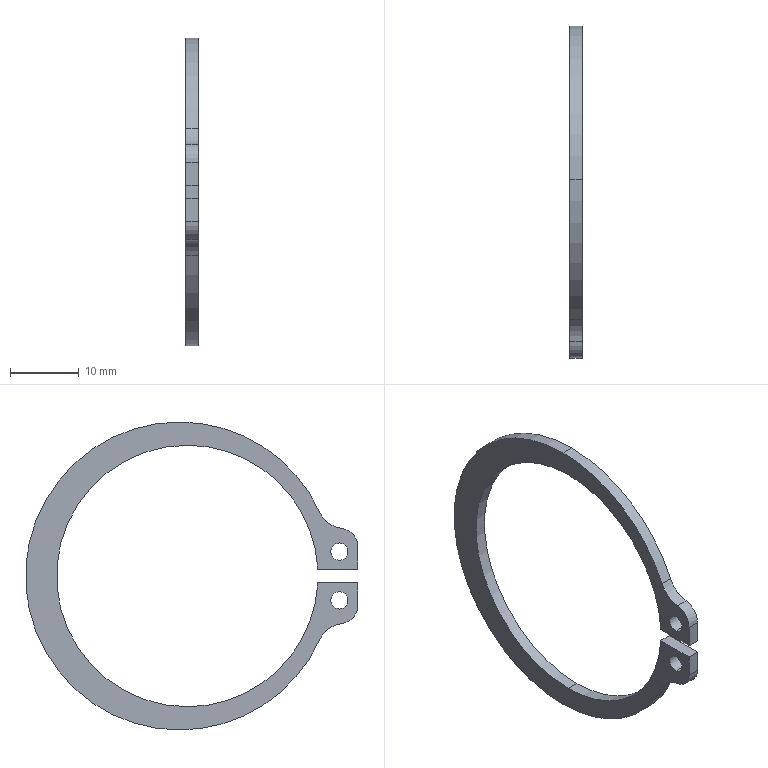Part | STEP file | SceondSTWN40_Default | 1 solid | 20 faces | box 1.75 x 48.3 x 44.75 mm | volume 824.122 mm3 | cylinder 14 | plane 6 | commonest cylinder face diameters 2.5 x4 38 x3 44.75 x3 5.4 x2 8.1 x2